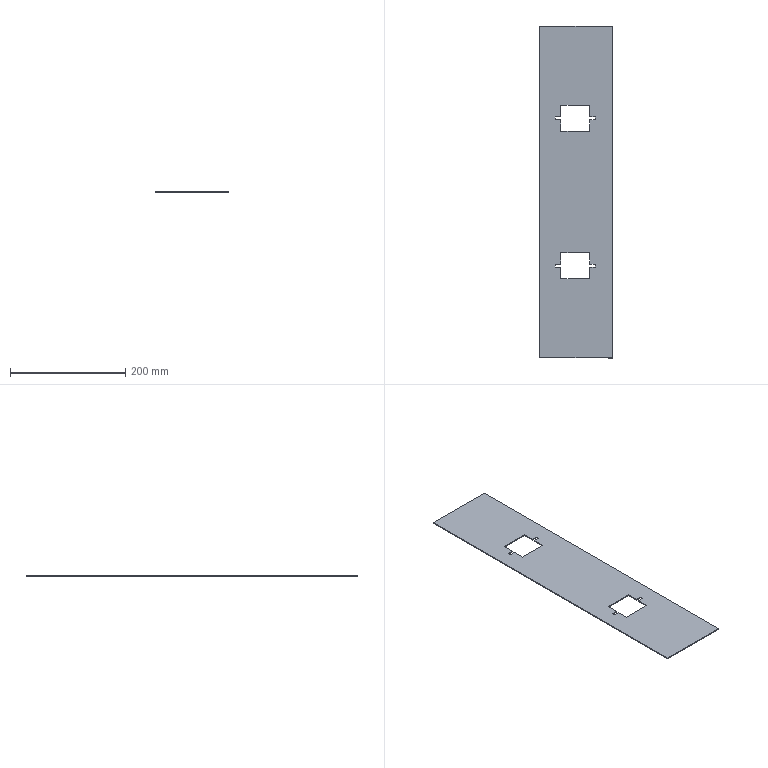Part | SolidWorks | features FlatPattern 1, SMBaseFlange 1, SheetMetal 1 | 1 solid | 30 faces | box 125 x 575 x 1.6 mm | volume 107480 mm3 | plane 30
STEP:
#1=CARTESIAN_POINT('',(-139.19,287.5,1.6));
#2=VERTEX_POINT('',#1);
#3=CARTESIAN_POINT('',(-139.19,-287.5,1.6));
#4=VERTEX_POINT('',#3);
#5=CARTESIAN_POINT('',(-139.19,287.5,1.6));
#6=DIRECTION('',(0.,-1.,0.));
#7=VECTOR('',#6,1000.);
#8=LINE('',#5,#7);
#9=EDGE_CURVE('',#2,#4,#8,.T.);
#10=ORIENTED_EDGE('',*,*,#9,.T.);
#11=CARTESIAN_POINT('',(-14.19,-287.5,1.6));
#12=VERTEX_POINT('',#11);
#13=CARTESIAN_POINT('',(-139.19,-287.5,1.6));
#14=DIRECTION('',(1.,0.,0.));
#15=VECTOR('',#14,1000.);
#16=LINE('',#13,#15);
#17=EDGE_CURVE('',#4,#12,#16,.T.);
#18=ORIENTED_EDGE('',*,*,#17,.T.);
#19=CARTESIAN_POINT('',(-14.19,287.5,1.6));
#20=VERTEX_POINT('',#19);
#21=CARTESIAN_POINT('',(-14.19,287.5,1.6));
#22=DIRECTION('',(0.,1.,0.));
#23=VECTOR('',#22,1000.);
#24=LINE('',#21,#23);
#25=EDGE_CURVE('',#12,#20,#24,.T.);
#26=ORIENTED_EDGE('',*,*,#25,.T.);
#27=CARTESIAN_POINT('',(-139.19,287.5,1.6));
#28=DIRECTION('',(-1.,0.,0.));
#29=VECTOR('',#28,1000.);
#30=LINE('',#27,#29);
#31=EDGE_CURVE('',#20,#2,#30,.T.);
#32=ORIENTED_EDGE('',*,*,#31,.T.);
#33=EDGE_LOOP('',(#10,#18,#26,#32));
#34=FACE_OUTER_BOUND('',#33,.T.);
#35=CARTESIAN_POINT('',(-113.004,-130.,1.6));
#36=VERTEX_POINT('',#35);
#37=CARTESIAN_POINT('',(-103.004,-130.,1.6));
#38=VERTEX_POINT('',#37);
#39=CARTESIAN_POINT('',(-113.004,-130.,1.6));
#40=DIRECTION('',(1.,0.,0.));
#41=VECTOR('',#40,1000.);
#42=LINE('',#39,#41);
#43=EDGE_CURVE('',#36,#38,#42,.T.);
#44=ORIENTED_EDGE('',*,*,#43,.F.);
#45=CARTESIAN_POINT('',(-113.004,-125.,1.6));
#46=VERTEX_POINT('',#45);
#47=CARTESIAN_POINT('',(-113.004,-125.,1.6));
#48=DIRECTION('',(0.,-1.,0.));
#49=VECTOR('',#48,1000.);
#50=LINE('',#47,#49);
#51=EDGE_CURVE('',#46,#36,#50,.T.);
#52=ORIENTED_EDGE('',*,*,#51,.F.);
#53=CARTESIAN_POINT('',(-103.004,-125.,1.6));
#54=VERTEX_POINT('',#53);
#55=CARTESIAN_POINT('',(-113.004,-125.,1.6));
#56=DIRECTION('',(-1.,0.,0.));
#57=VECTOR('',#56,1000.);
#58=LINE('',#55,#57);
#59=EDGE_CURVE('',#54,#46,#58,.T.);
#60=ORIENTED_EDGE('',*,*,#59,.F.);
#61=CARTESIAN_POINT('',(-103.004,-105.,1.6));
#62=VERTEX_POINT('',#61);
#63=CARTESIAN_POINT('',(-103.004,-105.,1.6));
#64=DIRECTION('',(0.,-1.,0.));
#65=VECTOR('',#64,1000.);
#66=LINE('',#63,#65);
#67=EDGE_CURVE('',#62,#54,#66,.T.);
#68=ORIENTED_EDGE('',*,*,#67,.F.);
#69=CARTESIAN_POINT('',(-53.004,-105.,1.6));
#70=VERTEX_POINT('',#69);
#71=CARTESIAN_POINT('',(-103.004,-105.,1.6));
#72=DIRECTION('',(-1.,0.,0.));
#73=VECTOR('',#72,1000.);
#74=LINE('',#71,#73);
#75=EDGE_CURVE('',#70,#62,#74,.T.);
#76=ORIENTED_EDGE('',*,*,#75,.F.);
#77=CARTESIAN_POINT('',(-53.004,-125.,1.6));
#78=VERTEX_POINT('',#77);
#79=CARTESIAN_POINT('',(-53.004,-105.,1.6));
#80=DIRECTION('',(0.,1.,0.));
#81=VECTOR('',#80,1000.);
#82=LINE('',#79,#81);
#83=EDGE_CURVE('',#78,#70,#82,.T.);
#84=ORIENTED_EDGE('',*,*,#83,.F.);
#85=CARTESIAN_POINT('',(-43.004,-125.,1.6));
#86=VERTEX_POINT('',#85);
#87=CARTESIAN_POINT('',(-53.004,-125.,1.6));
#88=DIRECTION('',(-1.,0.,0.));
#89=VECTOR('',#88,1000.);
#90=LINE('',#87,#89);
#91=EDGE_CURVE('',#86,#78,#90,.T.);
#92=ORIENTED_EDGE('',*,*,#91,.F.);
#93=CARTESIAN_POINT('',(-43.004,-130.,1.6));
#94=VERTEX_POINT('',#93);
#95=CARTESIAN_POINT('',(-43.004,-125.,1.6));
#96=DIRECTION('',(0.,1.,0.));
#97=VECTOR('',#96,1000.);
#98=LINE('',#95,#97);
#99=EDGE_CURVE('',#94,#86,#98,.T.);
#100=ORIENTED_EDGE('',*,*,#99,.F.);
#101=CARTESIAN_POINT('',(-53.004,-130.,1.6));
#102=VERTEX_POINT('',#101);
#103=CARTESIAN_POINT('',(-53.004,-130.,1.6));
#104=DIRECTION('',(1.,0.,0.));
#105=VECTOR('',#104,1000.);
#106=LINE('',#103,#105);
#107=EDGE_CURVE('',#102,#94,#106,.T.);
#108=ORIENTED_EDGE('',*,*,#107,.F.);
#109=CARTESIAN_POINT('',(-53.004,-150.,1.6));
#110=VERTEX_POINT('',#109);
#111=CARTESIAN_POINT('',(-53.004,-130.,1.6));
#112=DIRECTION('',(0.,1.,0.));
#113=VECTOR('',#112,1000.);
#114=LINE('',#111,#113);
#115=EDGE_CURVE('',#110,#102,#114,.T.);
#116=ORIENTED_EDGE('',*,*,#115,.F.);
#117=CARTESIAN_POINT('',(-103.004,-150.,1.6));
#118=VERTEX_POINT('',#117);
#119=CARTESIAN_POINT('',(-103.004,-150.,1.6));
#120=DIRECTION('',(1.,0.,0.));
#121=VECTOR('',#120,1000.);
#122=LINE('',#119,#121);
#123=EDGE_CURVE('',#118,#110,#122,.T.);
#124=ORIENTED_EDGE('',*,*,#123,.F.);
#125=CARTESIAN_POINT('',(-103.004,-130.,1.6));
#126=DIRECTION('',(0.,-1.,0.));
#127=VECTOR('',#126,1000.);
#128=LINE('',#125,#127);
#129=EDGE_CURVE('',#38,#118,#128,.T.);
#130=ORIENTED_EDGE('',*,*,#129,.F.);
#131=EDGE_LOOP('',(#44,#52,#60,#68,#76,#84,#92,#100,#108,#116,#124,#130));
#132=FACE_BOUND('',#131,.T.);
#133=CARTESIAN_POINT('',(-53.004,130.,1.6));
#134=VERTEX_POINT('',#133);
#135=CARTESIAN_POINT('',(-53.004,150.,1.6));
#136=VERTEX_POINT('',#135);
#137=CARTESIAN_POINT('',(-53.004,130.,1.6));
#138=DIRECTION('',(0.,1.,0.));
#139=VECTOR('',#138,1000.);
#140=LINE('',#137,#139);
#141=EDGE_CURVE('',#134,#136,#140,.T.);
#142=ORIENTED_EDGE('',*,*,#141,.F.);
#143=CARTESIAN_POINT('',(-43.004,130.,1.6));
#144=VERTEX_POINT('',#143);
#145=CARTESIAN_POINT('',(-53.004,130.,1.6));
#146=DIRECTION('',(-1.,0.,0.));
#147=VECTOR('',#146,1000.);
#148=LINE('',#145,#147);
#149=EDGE_CURVE('',#144,#134,#148,.T.);
#150=ORIENTED_EDGE('',*,*,#149,.F.);
#151=CARTESIAN_POINT('',(-43.004,125.,1.6));
#152=VERTEX_POINT('',#151);
#153=CARTESIAN_POINT('',(-43.004,125.,1.6));
#154=DIRECTION('',(0.,1.,0.));
#155=VECTOR('',#154,1000.);
#156=LINE('',#153,#155);
#157=EDGE_CURVE('',#152,#144,#156,.T.);
#158=ORIENTED_EDGE('',*,*,#157,.F.);
#159=CARTESIAN_POINT('',(-53.004,125.,1.6));
#160=VERTEX_POINT('',#159);
#161=CARTESIAN_POINT('',(-53.004,125.,1.6));
#162=DIRECTION('',(1.,0.,0.));
#163=VECTOR('',#162,1000.);
#164=LINE('',#161,#163);
#165=EDGE_CURVE('',#160,#152,#164,.T.);
#166=ORIENTED_EDGE('',*,*,#165,.F.);
#167=CARTESIAN_POINT('',(-53.004,105.,1.6));
#168=VERTEX_POINT('',#167);
#169=CARTESIAN_POINT('',(-53.004,105.,1.6));
#170=DIRECTION('',(0.,1.,0.));
#171=VECTOR('',#170,1000.);
#172=LINE('',#169,#171);
#173=EDGE_CURVE('',#168,#160,#172,.T.);
#174=ORIENTED_EDGE('',*,*,#173,.F.);
#175=CARTESIAN_POINT('',(-103.004,105.,1.6));
#176=VERTEX_POINT('',#175);
#177=CARTESIAN_POINT('',(-103.004,105.,1.6));
#178=DIRECTION('',(1.,0.,0.));
#179=VECTOR('',#178,1000.);
#180=LINE('',#177,#179);
#181=EDGE_CURVE('',#176,#168,#180,.T.);
#182=ORIENTED_EDGE('',*,*,#181,.F.);
#183=CARTESIAN_POINT('',(-103.004,125.,1.6));
#184=VERTEX_POINT('',#183);
#185=CARTESIAN_POINT('',(-103.004,105.,1.6));
#186=DIRECTION('',(0.,-1.,0.));
#187=VECTOR('',#186,1000.);
#188=LINE('',#185,#187);
#189=EDGE_CURVE('',#184,#176,#188,.T.);
#190=ORIENTED_EDGE('',*,*,#189,.F.);
#191=CARTESIAN_POINT('',(-113.004,125.,1.6));
#192=VERTEX_POINT('',#191);
#193=CARTESIAN_POINT('',(-113.004,125.,1.6));
#194=DIRECTION('',(1.,0.,0.));
#195=VECTOR('',#194,1000.);
#196=LINE('',#193,#195);
#197=EDGE_CURVE('',#192,#184,#196,.T.);
#198=ORIENTED_EDGE('',*,*,#197,.F.);
#199=CARTESIAN_POINT('',(-113.004,130.,1.6));
#200=VERTEX_POINT('',#199);
#201=CARTESIAN_POINT('',(-113.004,125.,1.6));
#202=DIRECTION('',(0.,-1.,0.));
#203=VECTOR('',#202,1000.);
#204=LINE('',#201,#203);
#205=EDGE_CURVE('',#200,#192,#204,.T.);
#206=ORIENTED_EDGE('',*,*,#205,.F.);
#207=CARTESIAN_POINT('',(-103.004,130.,1.6));
#208=VERTEX_POINT('',#207);
#209=CARTESIAN_POINT('',(-113.004,130.,1.6));
#210=DIRECTION('',(-1.,0.,0.));
#211=VECTOR('',#210,1000.);
#212=LINE('',#209,#211);
#213=EDGE_CURVE('',#208,#200,#212,.T.);
#214=ORIENTED_EDGE('',*,*,#213,.F.);
#215=CARTESIAN_POINT('',(-103.004,150.,1.6));
#216=VERTEX_POINT('',#215);
#217=CARTESIAN_POINT('',(-103.004,130.,1.6));
#218=DIRECTION('',(0.,-1.,0.));
#219=VECTOR('',#218,1000.);
#220=LINE('',#217,#219);
#221=EDGE_CURVE('',#216,#208,#220,.T.);
#222=ORIENTED_EDGE('',*,*,#221,.F.);
#223=CARTESIAN_POINT('',(-103.004,150.,1.6));
#224=DIRECTION('',(-1.,0.,0.));
#225=VECTOR('',#224,1000.);
#226=LINE('',#223,#225);
#227=EDGE_CURVE('',#136,#216,#226,.T.);
#228=ORIENTED_EDGE('',*,*,#227,.F.);
#229=EDGE_LOOP('',(#142,#150,#158,#166,#174,#182,#190,#198,#206,#214,#222,#228));
#230=FACE_BOUND('',#229,.T.);
#231=CARTESIAN_POINT('',(0.,0.,1.6));
#232=DIRECTION('',(0.,0.,1.));
#233=DIRECTION('',(1.,0.,0.));
#234=AXIS2_PLACEMENT_3D('',#231,#232,#233);
#235=PLANE('',#234);
#236=ADVANCED_FACE('',(#34,#132,#230),#235,.T.);
#237=CARTESIAN_POINT('',(-113.004,-125.,0.));
#238=VERTEX_POINT('',#237);
#239=CARTESIAN_POINT('',(-113.004,-130.,0.));
#240=VERTEX_POINT('',#239);
#241=CARTESIAN_POINT('',(-113.004,-125.,0.));
#242=DIRECTION('',(0.,-1.,0.));
#243=VECTOR('',#242,1000.);
#244=LINE('',#241,#243);
#245=EDGE_CURVE('',#238,#240,#244,.T.);
#246=ORIENTED_EDGE('',*,*,#245,.T.);
#247=CARTESIAN_POINT('',(-103.004,-130.,0.));
#248=VERTEX_POINT('',#247);
#249=CARTESIAN_POINT('',(-113.004,-130.,0.));
#250=DIRECTION('',(1.,0.,0.));
#251=VECTOR('',#250,1000.);
#252=LINE('',#249,#251);
#253=EDGE_CURVE('',#240,#248,#252,.T.);
#254=ORIENTED_EDGE('',*,*,#253,.T.);
#255=CARTESIAN_POINT('',(-103.004,-150.,0.));
#256=VERTEX_POINT('',#255);
#257=CARTESIAN_POINT('',(-103.004,-130.,0.));
#258=DIRECTION('',(0.,-1.,0.));
#259=VECTOR('',#258,1000.);
#260=LINE('',#257,#259);
#261=EDGE_CURVE('',#248,#256,#260,.T.);
#262=ORIENTED_EDGE('',*,*,#261,.T.);
#263=CARTESIAN_POINT('',(-53.004,-150.,0.));
#264=VERTEX_POINT('',#263);
#265=CARTESIAN_POINT('',(-103.004,-150.,0.));
#266=DIRECTION('',(1.,0.,0.));
#267=VECTOR('',#266,1000.);
#268=LINE('',#265,#267);
#269=EDGE_CURVE('',#256,#264,#268,.T.);
#270=ORIENTED_EDGE('',*,*,#269,.T.);
#271=CARTESIAN_POINT('',(-53.004,-130.,0.));
#272=VERTEX_POINT('',#271);
#273=CARTESIAN_POINT('',(-53.004,-130.,0.));
#274=DIRECTION('',(0.,1.,0.));
#275=VECTOR('',#274,1000.);
#276=LINE('',#273,#275);
#277=EDGE_CURVE('',#264,#272,#276,.T.);
#278=ORIENTED_EDGE('',*,*,#277,.T.);
#279=CARTESIAN_POINT('',(-43.004,-130.,0.));
#280=VERTEX_POINT('',#279);
#281=CARTESIAN_POINT('',(-53.004,-130.,0.));
#282=DIRECTION('',(1.,0.,0.));
#283=VECTOR('',#282,1000.);
#284=LINE('',#281,#283);
#285=EDGE_CURVE('',#272,#280,#284,.T.);
#286=ORIENTED_EDGE('',*,*,#285,.T.);
#287=CARTESIAN_POINT('',(-43.004,-125.,0.));
#288=VERTEX_POINT('',#287);
#289=CARTESIAN_POINT('',(-43.004,-125.,0.));
#290=DIRECTION('',(0.,1.,0.));
#291=VECTOR('',#290,1000.);
#292=LINE('',#289,#291);
#293=EDGE_CURVE('',#280,#288,#292,.T.);
#294=ORIENTED_EDGE('',*,*,#293,.T.);
#295=CARTESIAN_POINT('',(-53.004,-125.,0.));
#296=VERTEX_POINT('',#295);
#297=CARTESIAN_POINT('',(-53.004,-125.,0.));
#298=DIRECTION('',(-1.,0.,0.));
#299=VECTOR('',#298,1000.);
#300=LINE('',#297,#299);
#301=EDGE_CURVE('',#288,#296,#300,.T.);
#302=ORIENTED_EDGE('',*,*,#301,.T.);
#303=CARTESIAN_POINT('',(-53.004,-105.,0.));
#304=VERTEX_POINT('',#303);
#305=CARTESIAN_POINT('',(-53.004,-105.,0.));
#306=DIRECTION('',(0.,1.,0.));
#307=VECTOR('',#306,1000.);
#308=LINE('',#305,#307);
#309=EDGE_CURVE('',#296,#304,#308,.T.);
#310=ORIENTED_EDGE('',*,*,#309,.T.);
#311=CARTESIAN_POINT('',(-103.004,-105.,0.));
#312=VERTEX_POINT('',#311);
#313=CARTESIAN_POINT('',(-103.004,-105.,0.));
#314=DIRECTION('',(-1.,0.,0.));
#315=VECTOR('',#314,1000.);
#316=LINE('',#313,#315);
#317=EDGE_CURVE('',#304,#312,#316,.T.);
#318=ORIENTED_EDGE('',*,*,#317,.T.);
#319=CARTESIAN_POINT('',(-103.004,-125.,0.));
#320=VERTEX_POINT('',#319);
#321=CARTESIAN_POINT('',(-103.004,-105.,0.));
#322=DIRECTION('',(0.,-1.,0.));
#323=VECTOR('',#322,1000.);
#324=LINE('',#321,#323);
#325=EDGE_CURVE('',#312,#320,#324,.T.);
#326=ORIENTED_EDGE('',*,*,#325,.T.);
#327=CARTESIAN_POINT('',(-113.004,-125.,0.));
#328=DIRECTION('',(-1.,0.,0.));
#329=VECTOR('',#328,1000.);
#330=LINE('',#327,#329);
#331=EDGE_CURVE('',#320,#238,#330,.T.);
#332=ORIENTED_EDGE('',*,*,#331,.T.);
#333=EDGE_LOOP('',(#246,#254,#262,#270,#278,#286,#294,#302,#310,#318,#326,#332));
#334=FACE_BOUND('',#333,.T.);
#335=CARTESIAN_POINT('',(-139.19,287.5,0.));
#336=VERTEX_POINT('',#335);
#337=CARTESIAN_POINT('',(-139.19,-287.5,0.));
#338=VERTEX_POINT('',#337);
#339=CARTESIAN_POINT('',(-139.19,287.5,0.));
#340=DIRECTION('',(0.,-1.,0.));
#341=VECTOR('',#340,1000.);
#342=LINE('',#339,#341);
#343=EDGE_CURVE('',#336,#338,#342,.T.);
#344=ORIENTED_EDGE('',*,*,#343,.F.);
#345=CARTESIAN_POINT('',(-14.19,287.5,0.));
#346=VERTEX_POINT('',#345);
#347=CARTESIAN_POINT('',(-139.19,287.5,0.));
#348=DIRECTION('',(-1.,0.,0.));
#349=VECTOR('',#348,1000.);
#350=LINE('',#347,#349);
#351=EDGE_CURVE('',#346,#336,#350,.T.);
#352=ORIENTED_EDGE('',*,*,#351,.F.);
#353=CARTESIAN_POINT('',(-14.19,-287.5,0.));
#354=VERTEX_POINT('',#353);
#355=CARTESIAN_POINT('',(-14.19,287.5,0.));
#356=DIRECTION('',(0.,1.,0.));
#357=VECTOR('',#356,1000.);
#358=LINE('',#355,#357);
#359=EDGE_CURVE('',#354,#346,#358,.T.);
#360=ORIENTED_EDGE('',*,*,#359,.F.);
#361=CARTESIAN_POINT('',(-139.19,-287.5,0.));
#362=DIRECTION('',(1.,0.,0.));
#363=VECTOR('',#362,1000.);
#364=LINE('',#361,#363);
#365=EDGE_CURVE('',#338,#354,#364,.T.);
#366=ORIENTED_EDGE('',*,*,#365,.F.);
#367=EDGE_LOOP('',(#344,#352,#360,#366));
#368=FACE_OUTER_BOUND('',#367,.T.);
#369=CARTESIAN_POINT('',(-43.004,130.,0.));
#370=VERTEX_POINT('',#369);
#371=CARTESIAN_POINT('',(-53.004,130.,0.));
#372=VERTEX_POINT('',#371);
#373=CARTESIAN_POINT('',(-53.004,130.,0.));
#374=DIRECTION('',(-1.,0.,0.));
#375=VECTOR('',#374,1000.);
#376=LINE('',#373,#375);
#377=EDGE_CURVE('',#370,#372,#376,.T.);
#378=ORIENTED_EDGE('',*,*,#377,.T.);
#379=CARTESIAN_POINT('',(-53.004,150.,0.));
#380=VERTEX_POINT('',#379);
#381=CARTESIAN_POINT('',(-53.004,130.,0.));
#382=DIRECTION('',(0.,1.,0.));
#383=VECTOR('',#382,1000.);
#384=LINE('',#381,#383);
#385=EDGE_CURVE('',#372,#380,#384,.T.);
#386=ORIENTED_EDGE('',*,*,#385,.T.);
#387=CARTESIAN_POINT('',(-103.004,150.,0.));
#388=VERTEX_POINT('',#387);
#389=CARTESIAN_POINT('',(-103.004,150.,0.));
#390=DIRECTION('',(-1.,0.,0.));
#391=VECTOR('',#390,1000.);
#392=LINE('',#389,#391);
#393=EDGE_CURVE('',#380,#388,#392,.T.);
#394=ORIENTED_EDGE('',*,*,#393,.T.);
#395=CARTESIAN_POINT('',(-103.004,130.,0.));
#396=VERTEX_POINT('',#395);
#397=CARTESIAN_POINT('',(-103.004,130.,0.));
#398=DIRECTION('',(0.,-1.,0.));
#399=VECTOR('',#398,1000.);
#400=LINE('',#397,#399);
#401=EDGE_CURVE('',#388,#396,#400,.T.);
#402=ORIENTED_EDGE('',*,*,#401,.T.);
#403=CARTESIAN_POINT('',(-113.004,130.,0.));
#404=VERTEX_POINT('',#403);
#405=CARTESIAN_POINT('',(-113.004,130.,0.));
#406=DIRECTION('',(-1.,0.,0.));
#407=VECTOR('',#406,1000.);
#408=LINE('',#405,#407);
#409=EDGE_CURVE('',#396,#404,#408,.T.);
#410=ORIENTED_EDGE('',*,*,#409,.T.);
#411=CARTESIAN_POINT('',(-113.004,125.,0.));
#412=VERTEX_POINT('',#411);
#413=CARTESIAN_POINT('',(-113.004,125.,0.));
#414=DIRECTION('',(0.,-1.,0.));
#415=VECTOR('',#414,1000.);
#416=LINE('',#413,#415);
#417=EDGE_CURVE('',#404,#412,#416,.T.);
#418=ORIENTED_EDGE('',*,*,#417,.T.);
#419=CARTESIAN_POINT('',(-103.004,125.,0.));
#420=VERTEX_POINT('',#419);
#421=CARTESIAN_POINT('',(-113.004,125.,0.));
#422=DIRECTION('',(1.,0.,0.));
#423=VECTOR('',#422,1000.);
#424=LINE('',#421,#423);
#425=EDGE_CURVE('',#412,#420,#424,.T.);
#426=ORIENTED_EDGE('',*,*,#425,.T.);
#427=CARTESIAN_POINT('',(-103.004,105.,0.));
#428=VERTEX_POINT('',#427);
#429=CARTESIAN_POINT('',(-103.004,105.,0.));
#430=DIRECTION('',(0.,-1.,0.));
#431=VECTOR('',#430,1000.);
#432=LINE('',#429,#431);
#433=EDGE_CURVE('',#420,#428,#432,.T.);
#434=ORIENTED_EDGE('',*,*,#433,.T.);
#435=CARTESIAN_POINT('',(-53.004,105.,0.));
#436=VERTEX_POINT('',#435);
#437=CARTESIAN_POINT('',(-103.004,105.,0.));
#438=DIRECTION('',(1.,0.,0.));
#439=VECTOR('',#438,1000.);
#440=LINE('',#437,#439);
#441=EDGE_CURVE('',#428,#436,#440,.T.);
#442=ORIENTED_EDGE('',*,*,#441,.T.);
#443=CARTESIAN_POINT('',(-53.004,125.,0.));
#444=VERTEX_POINT('',#443);
#445=CARTESIAN_POINT('',(-53.004,105.,0.));
#446=DIRECTION('',(0.,1.,0.));
#447=VECTOR('',#446,1000.);
#448=LINE('',#445,#447);
#449=EDGE_CURVE('',#436,#444,#448,.T.);
#450=ORIENTED_EDGE('',*,*,#449,.T.);
#451=CARTESIAN_POINT('',(-43.004,125.,0.));
#452=VERTEX_POINT('',#451);
#453=CARTESIAN_POINT('',(-53.004,125.,0.));
#454=DIRECTION('',(1.,0.,0.));
#455=VECTOR('',#454,1000.);
#456=LINE('',#453,#455);
#457=EDGE_CURVE('',#444,#452,#456,.T.);
#458=ORIENTED_EDGE('',*,*,#457,.T.);
#459=CARTESIAN_POINT('',(-43.004,125.,0.));
#460=DIRECTION('',(0.,1.,0.));
#461=VECTOR('',#460,1000.);
#462=LINE('',#459,#461);
#463=EDGE_CURVE('',#452,#370,#462,.T.);
#464=ORIENTED_EDGE('',*,*,#463,.T.);
#465=EDGE_LOOP('',(#378,#386,#394,#402,#410,#418,#426,#434,#442,#450,#458,#464));
#466=FACE_BOUND('',#465,.T.);
#467=CARTESIAN_POINT('',(0.,0.,0.));
#468=DIRECTION('',(0.,0.,1.));
#469=DIRECTION('',(1.,0.,0.));
#470=AXIS2_PLACEMENT_3D('',#467,#468,#469);
#471=PLANE('',#470);
#472=ADVANCED_FACE('',(#334,#368,#466),#471,.F.);
#473=ORIENTED_EDGE('',*,*,#343,.T.);
#474=CARTESIAN_POINT('',(-139.19,-287.5,1.6));
#475=DIRECTION('',(0.,0.,-1.));
#476=VECTOR('',#475,1000.);
#477=LINE('',#474,#476);
#478=EDGE_CURVE('',#4,#338,#477,.T.);
#479=ORIENTED_EDGE('',*,*,#478,.F.);
#480=ORIENTED_EDGE('',*,*,#9,.F.);
#481=CARTESIAN_POINT('',(-139.19,287.5,1.6));
#482=DIRECTION('',(0.,0.,-1.));
#483=VECTOR('',#482,1000.);
#484=LINE('',#481,#483);
#485=EDGE_CURVE('',#2,#336,#484,.T.);
#486=ORIENTED_EDGE('',*,*,#485,.T.);
#487=EDGE_LOOP('',(#473,#479,#480,#486));
#488=FACE_OUTER_BOUND('',#487,.T.);
#489=CARTESIAN_POINT('',(-139.19,287.5,1.6));
#490=DIRECTION('',(1.,0.,0.));
#491=DIRECTION('',(0.,0.,-1.));
#492=AXIS2_PLACEMENT_3D('',#489,#490,#491);
#493=PLANE('',#492);
#494=ADVANCED_FACE('',(#488),#493,.F.);
#495=ORIENTED_EDGE('',*,*,#365,.T.);
#496=CARTESIAN_POINT('',(-14.19,-287.5,1.6));
#497=DIRECTION('',(0.,0.,-1.));
#498=VECTOR('',#497,1000.);
#499=LINE('',#496,#498);
#500=EDGE_CURVE('',#12,#354,#499,.T.);
#501=ORIENTED_EDGE('',*,*,#500,.F.);
#502=ORIENTED_EDGE('',*,*,#17,.F.);
#503=ORIENTED_EDGE('',*,*,#478,.T.);
#504=EDGE_LOOP('',(#495,#501,#502,#503));
#505=FACE_OUTER_BOUND('',#504,.T.);
#506=CARTESIAN_POINT('',(-139.19,-287.5,1.6));
#507=DIRECTION('',(0.,1.,0.));
#508=DIRECTION('',(-1.,0.,0.));
#509=AXIS2_PLACEMENT_3D('',#506,#507,#508);
#510=PLANE('',#509);
#511=ADVANCED_FACE('',(#505),#510,.F.);
#512=ORIENTED_EDGE('',*,*,#359,.T.);
#513=CARTESIAN_POINT('',(-14.19,287.5,1.6));
#514=DIRECTION('',(0.,0.,-1.));
#515=VECTOR('',#514,1000.);
#516=LINE('',#513,#515);
#517=EDGE_CURVE('',#20,#346,#516,.T.);
#518=ORIENTED_EDGE('',*,*,#517,.F.);
#519=ORIENTED_EDGE('',*,*,#25,.F.);
#520=ORIENTED_EDGE('',*,*,#500,.T.);
#521=EDGE_LOOP('',(#512,#518,#519,#520));
#522=FACE_OUTER_BOUND('',#521,.T.);
#523=CARTESIAN_POINT('',(-14.19,287.5,1.6));
#524=DIRECTION('',(-1.,0.,0.));
#525=DIRECTION('',(0.,-1.,0.));
#526=AXIS2_PLACEMENT_3D('',#523,#524,#525);
#527=PLANE('',#526);
#528=ADVANCED_FACE('',(#522),#527,.F.);
#529=ORIENTED_EDGE('',*,*,#351,.T.);
#530=ORIENTED_EDGE('',*,*,#485,.F.);
#531=ORIENTED_EDGE('',*,*,#31,.F.);
#532=ORIENTED_EDGE('',*,*,#517,.T.);
#533=EDGE_LOOP('',(#529,#530,#531,#532));
#534=FACE_OUTER_BOUND('',#533,.T.);
#535=CARTESIAN_POINT('',(-139.19,287.5,1.6));
#536=DIRECTION('',(0.,-1.,0.));
#537=DIRECTION('',(0.,0.,-1.));
#538=AXIS2_PLACEMENT_3D('',#535,#536,#537);
#539=PLANE('',#538);
#540=ADVANCED_FACE('',(#534),#539,.F.);
#541=ORIENTED_EDGE('',*,*,#245,.F.);
#542=CARTESIAN_POINT('',(-113.004,-125.,1.6));
#543=DIRECTION('',(0.,0.,-1.));
#544=VECTOR('',#543,1000.);
#545=LINE('',#542,#544);
#546=EDGE_CURVE('',#46,#238,#545,.T.);
#547=ORIENTED_EDGE('',*,*,#546,.F.);
#548=ORIENTED_EDGE('',*,*,#51,.T.);
#549=CARTESIAN_POINT('',(-113.004,-130.,1.6));
#550=DIRECTION('',(0.,0.,-1.));
#551=VECTOR('',#550,1000.);
#552=LINE('',#549,#551);
#553=EDGE_CURVE('',#36,#240,#552,.T.);
#554=ORIENTED_EDGE('',*,*,#553,.T.);
#555=EDGE_LOOP('',(#541,#547,#548,#554));
#556=FACE_OUTER_BOUND('',#555,.T.);
#557=CARTESIAN_POINT('',(-113.004,-125.,1.6));
#558=DIRECTION('',(1.,0.,0.));
#559=DIRECTION('',(0.,0.,-1.));
#560=AXIS2_PLACEMENT_3D('',#557,#558,#559);
#561=PLANE('',#560);
#562=ADVANCED_FACE('',(#556),#561,.T.);
#563=ORIENTED_EDGE('',*,*,#253,.F.);
#564=ORIENTED_EDGE('',*,*,#553,.F.);
#565=ORIENTED_EDGE('',*,*,#43,.T.);
#566=CARTESIAN_POINT('',(-103.004,-130.,1.6));
#567=DIRECTION('',(0.,0.,-1.));
#568=VECTOR('',#567,1000.);
#569=LINE('',#566,#568);
#570=EDGE_CURVE('',#38,#248,#569,.T.);
#571=ORIENTED_EDGE('',*,*,#570,.T.);
#572=EDGE_LOOP('',(#563,#564,#565,#571));
#573=FACE_OUTER_BOUND('',#572,.T.);
#574=CARTESIAN_POINT('',(-113.004,-130.,1.6));
#575=DIRECTION('',(0.,1.,0.));
#576=DIRECTION('',(0.,0.,1.));
#577=AXIS2_PLACEMENT_3D('',#574,#575,#576);
#578=PLANE('',#577);
#579=ADVANCED_FACE('',(#573),#578,.T.);
#580=ORIENTED_EDGE('',*,*,#261,.F.);
#581=ORIENTED_EDGE('',*,*,#570,.F.);
#582=ORIENTED_EDGE('',*,*,#129,.T.);
#583=CARTESIAN_POINT('',(-103.004,-150.,1.6));
#584=DIRECTION('',(0.,0.,-1.));
#585=VECTOR('',#584,1000.);
#586=LINE('',#583,#585);
#587=EDGE_CURVE('',#118,#256,#586,.T.);
#588=ORIENTED_EDGE('',*,*,#587,.T.);
#589=EDGE_LOOP('',(#580,#581,#582,#588));
#590=FACE_OUTER_BOUND('',#589,.T.);
#591=CARTESIAN_POINT('',(-103.004,-130.,1.6));
#592=DIRECTION('',(1.,0.,0.));
#593=DIRECTION('',(0.,0.,-1.));
#594=AXIS2_PLACEMENT_3D('',#591,#592,#593);
#595=PLANE('',#594);
#596=ADVANCED_FACE('',(#590),#595,.T.);
#597=ORIENTED_EDGE('',*,*,#269,.F.);
#598=ORIENTED_EDGE('',*,*,#587,.F.);
#599=ORIENTED_EDGE('',*,*,#123,.T.);
#600=CARTESIAN_POINT('',(-53.004,-150.,1.6));
#601=DIRECTION('',(0.,0.,-1.));
#602=VECTOR('',#601,1000.);
#603=LINE('',#600,#602);
#604=EDGE_CURVE('',#110,#264,#603,.T.);
#605=ORIENTED_EDGE('',*,*,#604,.T.);
#606=EDGE_LOOP('',(#597,#598,#599,#605));
#607=FACE_OUTER_BOUND('',#606,.T.);
#608=CARTESIAN_POINT('',(-103.004,-150.,1.6));
#609=DIRECTION('',(0.,1.,0.));
#610=DIRECTION('',(0.,0.,1.));
#611=AXIS2_PLACEMENT_3D('',#608,#609,#610);
#612=PLANE('',#611);
#613=ADVANCED_FACE('',(#607),#612,.T.);
#614=ORIENTED_EDGE('',*,*,#277,.F.);
#615=ORIENTED_EDGE('',*,*,#604,.F.);
#616=ORIENTED_EDGE('',*,*,#115,.T.);
#617=CARTESIAN_POINT('',(-53.004,-130.,1.6));
#618=DIRECTION('',(0.,0.,-1.));
#619=VECTOR('',#618,1000.);
#620=LINE('',#617,#619);
#621=EDGE_CURVE('',#102,#272,#620,.T.);
#622=ORIENTED_EDGE('',*,*,#621,.T.);
#623=EDGE_LOOP('',(#614,#615,#616,#622));
#624=FACE_OUTER_BOUND('',#623,.T.);
#625=CARTESIAN_POINT('',(-53.004,-130.,1.6));
#626=DIRECTION('',(-1.,0.,0.));
#627=DIRECTION('',(0.,0.,1.));
#628=AXIS2_PLACEMENT_3D('',#625,#626,#627);
#629=PLANE('',#628);
#630=ADVANCED_FACE('',(#624),#629,.T.);
#631=ORIENTED_EDGE('',*,*,#285,.F.);
#632=ORIENTED_EDGE('',*,*,#621,.F.);
#633=ORIENTED_EDGE('',*,*,#107,.T.);
#634=CARTESIAN_POINT('',(-43.004,-130.,1.6));
#635=DIRECTION('',(0.,0.,-1.));
#636=VECTOR('',#635,1000.);
#637=LINE('',#634,#636);
#638=EDGE_CURVE('',#94,#280,#637,.T.);
#639=ORIENTED_EDGE('',*,*,#638,.T.);
#640=EDGE_LOOP('',(#631,#632,#633,#639));
#641=FACE_OUTER_BOUND('',#640,.T.);
#642=CARTESIAN_POINT('',(-53.004,-130.,1.6));
#643=DIRECTION('',(0.,1.,0.));
#644=DIRECTION('',(0.,0.,1.));
#645=AXIS2_PLACEMENT_3D('',#642,#643,#644);
#646=PLANE('',#645);
#647=ADVANCED_FACE('',(#641),#646,.T.);
#648=ORIENTED_EDGE('',*,*,#293,.F.);
#649=ORIENTED_EDGE('',*,*,#638,.F.);
#650=ORIENTED_EDGE('',*,*,#99,.T.);
#651=CARTESIAN_POINT('',(-43.004,-125.,1.6));
#652=DIRECTION('',(0.,0.,-1.));
#653=VECTOR('',#652,1000.);
#654=LINE('',#651,#653);
#655=EDGE_CURVE('',#86,#288,#654,.T.);
#656=ORIENTED_EDGE('',*,*,#655,.T.);
#657=EDGE_LOOP('',(#648,#649,#650,#656));
#658=FACE_OUTER_BOUND('',#657,.T.);
#659=CARTESIAN_POINT('',(-43.004,-125.,1.6));
#660=DIRECTION('',(-1.,0.,0.));
#661=DIRECTION('',(0.,0.,1.));
#662=AXIS2_PLACEMENT_3D('',#659,#660,#661);
#663=PLANE('',#662);
#664=ADVANCED_FACE('',(#658),#663,.T.);
#665=ORIENTED_EDGE('',*,*,#301,.F.);
#666=ORIENTED_EDGE('',*,*,#655,.F.);
#667=ORIENTED_EDGE('',*,*,#91,.T.);
#668=CARTESIAN_POINT('',(-53.004,-125.,1.6));
#669=DIRECTION('',(0.,0.,-1.));
#670=VECTOR('',#669,1000.);
#671=LINE('',#668,#670);
#672=EDGE_CURVE('',#78,#296,#671,.T.);
#673=ORIENTED_EDGE('',*,*,#672,.T.);
#674=EDGE_LOOP('',(#665,#666,#667,#673));
#675=FACE_OUTER_BOUND('',#674,.T.);
#676=CARTESIAN_POINT('',(-53.004,-125.,1.6));
#677=DIRECTION('',(0.,-1.,0.));
#678=DIRECTION('',(0.,0.,-1.));
#679=AXIS2_PLACEMENT_3D('',#676,#677,#678);
#680=PLANE('',#679);
#681=ADVANCED_FACE('',(#675),#680,.T.);
#682=ORIENTED_EDGE('',*,*,#309,.F.);
#683=ORIENTED_EDGE('',*,*,#672,.F.);
#684=ORIENTED_EDGE('',*,*,#83,.T.);
#685=CARTESIAN_POINT('',(-53.004,-105.,1.6));
#686=DIRECTION('',(0.,0.,-1.));
#687=VECTOR('',#686,1000.);
#688=LINE('',#685,#687);
#689=EDGE_CURVE('',#70,#304,#688,.T.);
#690=ORIENTED_EDGE('',*,*,#689,.T.);
#691=EDGE_LOOP('',(#682,#683,#684,#690));
#692=FACE_OUTER_BOUND('',#691,.T.);
#693=CARTESIAN_POINT('',(-53.004,-105.,1.6));
#694=DIRECTION('',(-1.,0.,0.));
#695=DIRECTION('',(0.,0.,1.));
#696=AXIS2_PLACEMENT_3D('',#693,#694,#695);
#697=PLANE('',#696);
#698=ADVANCED_FACE('',(#692),#697,.T.);
#699=ORIENTED_EDGE('',*,*,#317,.F.);
#700=ORIENTED_EDGE('',*,*,#689,.F.);
#701=ORIENTED_EDGE('',*,*,#75,.T.);
#702=CARTESIAN_POINT('',(-103.004,-105.,1.6));
#703=DIRECTION('',(0.,0.,-1.));
#704=VECTOR('',#703,1000.);
#705=LINE('',#702,#704);
#706=EDGE_CURVE('',#62,#312,#705,.T.);
#707=ORIENTED_EDGE('',*,*,#706,.T.);
#708=EDGE_LOOP('',(#699,#700,#701,#707));
#709=FACE_OUTER_BOUND('',#708,.T.);
#710=CARTESIAN_POINT('',(-103.004,-105.,1.6));
#711=DIRECTION('',(0.,-1.,0.));
#712=DIRECTION('',(0.,0.,-1.));
#713=AXIS2_PLACEMENT_3D('',#710,#711,#712);
#714=PLANE('',#713);
#715=ADVANCED_FACE('',(#709),#714,.T.);
#716=ORIENTED_EDGE('',*,*,#325,.F.);
#717=ORIENTED_EDGE('',*,*,#706,.F.);
#718=ORIENTED_EDGE('',*,*,#67,.T.);
#719=CARTESIAN_POINT('',(-103.004,-125.,1.6));
#720=DIRECTION('',(0.,0.,-1.));
#721=VECTOR('',#720,1000.);
#722=LINE('',#719,#721);
#723=EDGE_CURVE('',#54,#320,#722,.T.);
#724=ORIENTED_EDGE('',*,*,#723,.T.);
#725=EDGE_LOOP('',(#716,#717,#718,#724));
#726=FACE_OUTER_BOUND('',#725,.T.);
#727=CARTESIAN_POINT('',(-103.004,-105.,1.6));
#728=DIRECTION('',(1.,0.,0.));
#729=DIRECTION('',(0.,0.,-1.));
#730=AXIS2_PLACEMENT_3D('',#727,#728,#729);
#731=PLANE('',#730);
#732=ADVANCED_FACE('',(#726),#731,.T.);
#733=ORIENTED_EDGE('',*,*,#331,.F.);
#734=ORIENTED_EDGE('',*,*,#723,.F.);
#735=ORIENTED_EDGE('',*,*,#59,.T.);
#736=ORIENTED_EDGE('',*,*,#546,.T.);
#737=EDGE_LOOP('',(#733,#734,#735,#736));
#738=FACE_OUTER_BOUND('',#737,.T.);
#739=CARTESIAN_POINT('',(-113.004,-125.,1.6));
#740=DIRECTION('',(0.,-1.,0.));
#741=DIRECTION('',(0.,0.,-1.));
#742=AXIS2_PLACEMENT_3D('',#739,#740,#741);
#743=PLANE('',#742);
#744=ADVANCED_FACE('',(#738),#743,.T.);
#745=ORIENTED_EDGE('',*,*,#377,.F.);
#746=CARTESIAN_POINT('',(-43.004,130.,1.6));
#747=DIRECTION('',(0.,0.,-1.));
#748=VECTOR('',#747,1000.);
#749=LINE('',#746,#748);
#750=EDGE_CURVE('',#144,#370,#749,.T.);
#751=ORIENTED_EDGE('',*,*,#750,.F.);
#752=ORIENTED_EDGE('',*,*,#149,.T.);
#753=CARTESIAN_POINT('',(-53.004,130.,1.6));
#754=DIRECTION('',(0.,0.,-1.));
#755=VECTOR('',#754,1000.);
#756=LINE('',#753,#755);
#757=EDGE_CURVE('',#134,#372,#756,.T.);
#758=ORIENTED_EDGE('',*,*,#757,.T.);
#759=EDGE_LOOP('',(#745,#751,#752,#758));
#760=FACE_OUTER_BOUND('',#759,.T.);
#761=CARTESIAN_POINT('',(-53.004,130.,1.6));
#762=DIRECTION('',(0.,-1.,0.));
#763=DIRECTION('',(0.,0.,-1.));
#764=AXIS2_PLACEMENT_3D('',#761,#762,#763);
#765=PLANE('',#764);
#766=ADVANCED_FACE('',(#760),#765,.T.);
#767=ORIENTED_EDGE('',*,*,#385,.F.);
#768=ORIENTED_EDGE('',*,*,#757,.F.);
#769=ORIENTED_EDGE('',*,*,#141,.T.);
#770=CARTESIAN_POINT('',(-53.004,150.,1.6));
#771=DIRECTION('',(0.,0.,-1.));
#772=VECTOR('',#771,1000.);
#773=LINE('',#770,#772);
#774=EDGE_CURVE('',#136,#380,#773,.T.);
#775=ORIENTED_EDGE('',*,*,#774,.T.);
#776=EDGE_LOOP('',(#767,#768,#769,#775));
#777=FACE_OUTER_BOUND('',#776,.T.);
#778=CARTESIAN_POINT('',(-53.004,130.,1.6));
#779=DIRECTION('',(-1.,0.,0.));
#780=DIRECTION('',(0.,0.,1.));
#781=AXIS2_PLACEMENT_3D('',#778,#779,#780);
#782=PLANE('',#781);
#783=ADVANCED_FACE('',(#777),#782,.T.);
#784=ORIENTED_EDGE('',*,*,#393,.F.);
#785=ORIENTED_EDGE('',*,*,#774,.F.);
#786=ORIENTED_EDGE('',*,*,#227,.T.);
#787=CARTESIAN_POINT('',(-103.004,150.,1.6));
#788=DIRECTION('',(0.,0.,-1.));
#789=VECTOR('',#788,1000.);
#790=LINE('',#787,#789);
#791=EDGE_CURVE('',#216,#388,#790,.T.);
#792=ORIENTED_EDGE('',*,*,#791,.T.);
#793=EDGE_LOOP('',(#784,#785,#786,#792));
#794=FACE_OUTER_BOUND('',#793,.T.);
#795=CARTESIAN_POINT('',(-103.004,150.,1.6));
#796=DIRECTION('',(0.,-1.,0.));
#797=DIRECTION('',(0.,0.,-1.));
#798=AXIS2_PLACEMENT_3D('',#795,#796,#797);
#799=PLANE('',#798);
#800=ADVANCED_FACE('',(#794),#799,.T.);
#801=ORIENTED_EDGE('',*,*,#401,.F.);
#802=ORIENTED_EDGE('',*,*,#791,.F.);
#803=ORIENTED_EDGE('',*,*,#221,.T.);
#804=CARTESIAN_POINT('',(-103.004,130.,1.6));
#805=DIRECTION('',(0.,0.,-1.));
#806=VECTOR('',#805,1000.);
#807=LINE('',#804,#806);
#808=EDGE_CURVE('',#208,#396,#807,.T.);
#809=ORIENTED_EDGE('',*,*,#808,.T.);
#810=EDGE_LOOP('',(#801,#802,#803,#809));
#811=FACE_OUTER_BOUND('',#810,.T.);
#812=CARTESIAN_POINT('',(-103.004,130.,1.6));
#813=DIRECTION('',(1.,0.,0.));
#814=DIRECTION('',(0.,0.,-1.));
#815=AXIS2_PLACEMENT_3D('',#812,#813,#814);
#816=PLANE('',#815);
#817=ADVANCED_FACE('',(#811),#816,.T.);
#818=ORIENTED_EDGE('',*,*,#409,.F.);
#819=ORIENTED_EDGE('',*,*,#808,.F.);
#820=ORIENTED_EDGE('',*,*,#213,.T.);
#821=CARTESIAN_POINT('',(-113.004,130.,1.6));
#822=DIRECTION('',(0.,0.,-1.));
#823=VECTOR('',#822,1000.);
#824=LINE('',#821,#823);
#825=EDGE_CURVE('',#200,#404,#824,.T.);
#826=ORIENTED_EDGE('',*,*,#825,.T.);
#827=EDGE_LOOP('',(#818,#819,#820,#826));
#828=FACE_OUTER_BOUND('',#827,.T.);
#829=CARTESIAN_POINT('',(-113.004,130.,1.6));
#830=DIRECTION('',(0.,-1.,0.));
#831=DIRECTION('',(0.,0.,-1.));
#832=AXIS2_PLACEMENT_3D('',#829,#830,#831);
#833=PLANE('',#832);
#834=ADVANCED_FACE('',(#828),#833,.T.);
#835=ORIENTED_EDGE('',*,*,#417,.F.);
#836=ORIENTED_EDGE('',*,*,#825,.F.);
#837=ORIENTED_EDGE('',*,*,#205,.T.);
#838=CARTESIAN_POINT('',(-113.004,125.,1.6));
#839=DIRECTION('',(0.,0.,-1.));
#840=VECTOR('',#839,1000.);
#841=LINE('',#838,#840);
#842=EDGE_CURVE('',#192,#412,#841,.T.);
#843=ORIENTED_EDGE('',*,*,#842,.T.);
#844=EDGE_LOOP('',(#835,#836,#837,#843));
#845=FACE_OUTER_BOUND('',#844,.T.);
#846=CARTESIAN_POINT('',(-113.004,125.,1.6));
#847=DIRECTION('',(1.,0.,0.));
#848=DIRECTION('',(0.,0.,-1.));
#849=AXIS2_PLACEMENT_3D('',#846,#847,#848);
#850=PLANE('',#849);
#851=ADVANCED_FACE('',(#845),#850,.T.);
#852=ORIENTED_EDGE('',*,*,#425,.F.);
#853=ORIENTED_EDGE('',*,*,#842,.F.);
#854=ORIENTED_EDGE('',*,*,#197,.T.);
#855=CARTESIAN_POINT('',(-103.004,125.,1.6));
#856=DIRECTION('',(0.,0.,-1.));
#857=VECTOR('',#856,1000.);
#858=LINE('',#855,#857);
#859=EDGE_CURVE('',#184,#420,#858,.T.);
#860=ORIENTED_EDGE('',*,*,#859,.T.);
#861=EDGE_LOOP('',(#852,#853,#854,#860));
#862=FACE_OUTER_BOUND('',#861,.T.);
#863=CARTESIAN_POINT('',(-113.004,125.,1.6));
#864=DIRECTION('',(0.,1.,0.));
#865=DIRECTION('',(0.,0.,1.));
#866=AXIS2_PLACEMENT_3D('',#863,#864,#865);
#867=PLANE('',#866);
#868=ADVANCED_FACE('',(#862),#867,.T.);
#869=ORIENTED_EDGE('',*,*,#433,.F.);
#870=ORIENTED_EDGE('',*,*,#859,.F.);
#871=ORIENTED_EDGE('',*,*,#189,.T.);
#872=CARTESIAN_POINT('',(-103.004,105.,1.6));
#873=DIRECTION('',(0.,0.,-1.));
#874=VECTOR('',#873,1000.);
#875=LINE('',#872,#874);
#876=EDGE_CURVE('',#176,#428,#875,.T.);
#877=ORIENTED_EDGE('',*,*,#876,.T.);
#878=EDGE_LOOP('',(#869,#870,#871,#877));
#879=FACE_OUTER_BOUND('',#878,.T.);
#880=CARTESIAN_POINT('',(-103.004,105.,1.6));
#881=DIRECTION('',(1.,0.,0.));
#882=DIRECTION('',(0.,0.,-1.));
#883=AXIS2_PLACEMENT_3D('',#880,#881,#882);
#884=PLANE('',#883);
#885=ADVANCED_FACE('',(#879),#884,.T.);
#886=ORIENTED_EDGE('',*,*,#441,.F.);
#887=ORIENTED_EDGE('',*,*,#876,.F.);
#888=ORIENTED_EDGE('',*,*,#181,.T.);
#889=CARTESIAN_POINT('',(-53.004,105.,1.6));
#890=DIRECTION('',(0.,0.,-1.));
#891=VECTOR('',#890,1000.);
#892=LINE('',#889,#891);
#893=EDGE_CURVE('',#168,#436,#892,.T.);
#894=ORIENTED_EDGE('',*,*,#893,.T.);
#895=EDGE_LOOP('',(#886,#887,#888,#894));
#896=FACE_OUTER_BOUND('',#895,.T.);
#897=CARTESIAN_POINT('',(-103.004,105.,1.6));
#898=DIRECTION('',(0.,1.,0.));
#899=DIRECTION('',(0.,0.,1.));
#900=AXIS2_PLACEMENT_3D('',#897,#898,#899);
#901=PLANE('',#900);
#902=ADVANCED_FACE('',(#896),#901,.T.);
#903=ORIENTED_EDGE('',*,*,#449,.F.);
#904=ORIENTED_EDGE('',*,*,#893,.F.);
#905=ORIENTED_EDGE('',*,*,#173,.T.);
#906=CARTESIAN_POINT('',(-53.004,125.,1.6));
#907=DIRECTION('',(0.,0.,-1.));
#908=VECTOR('',#907,1000.);
#909=LINE('',#906,#908);
#910=EDGE_CURVE('',#160,#444,#909,.T.);
#911=ORIENTED_EDGE('',*,*,#910,.T.);
#912=EDGE_LOOP('',(#903,#904,#905,#911));
#913=FACE_OUTER_BOUND('',#912,.T.);
#914=CARTESIAN_POINT('',(-53.004,105.,1.6));
#915=DIRECTION('',(-1.,0.,0.));
#916=DIRECTION('',(0.,0.,1.));
#917=AXIS2_PLACEMENT_3D('',#914,#915,#916);
#918=PLANE('',#917);
#919=ADVANCED_FACE('',(#913),#918,.T.);
#920=ORIENTED_EDGE('',*,*,#457,.F.);
#921=ORIENTED_EDGE('',*,*,#910,.F.);
#922=ORIENTED_EDGE('',*,*,#165,.T.);
#923=CARTESIAN_POINT('',(-43.004,125.,1.6));
#924=DIRECTION('',(0.,0.,-1.));
#925=VECTOR('',#924,1000.);
#926=LINE('',#923,#925);
#927=EDGE_CURVE('',#152,#452,#926,.T.);
#928=ORIENTED_EDGE('',*,*,#927,.T.);
#929=EDGE_LOOP('',(#920,#921,#922,#928));
#930=FACE_OUTER_BOUND('',#929,.T.);
#931=CARTESIAN_POINT('',(-53.004,125.,1.6));
#932=DIRECTION('',(0.,1.,0.));
#933=DIRECTION('',(0.,0.,1.));
#934=AXIS2_PLACEMENT_3D('',#931,#932,#933);
#935=PLANE('',#934);
#936=ADVANCED_FACE('',(#930),#935,.T.);
#937=ORIENTED_EDGE('',*,*,#463,.F.);
#938=ORIENTED_EDGE('',*,*,#927,.F.);
#939=ORIENTED_EDGE('',*,*,#157,.T.);
#940=ORIENTED_EDGE('',*,*,#750,.T.);
#941=EDGE_LOOP('',(#937,#938,#939,#940));
#942=FACE_OUTER_BOUND('',#941,.T.);
#943=CARTESIAN_POINT('',(-43.004,125.,1.6));
#944=DIRECTION('',(-1.,0.,0.));
#945=DIRECTION('',(0.,0.,1.));
#946=AXIS2_PLACEMENT_3D('',#943,#944,#945);
#947=PLANE('',#946);
#948=ADVANCED_FACE('',(#942),#947,.T.);
#949=CLOSED_SHELL('',(#236,#472,#494,#511,#528,#540,#562,#579,#596,#613,#630,#647,#664,#681,#698,#715,#732,#744,#766,#783,#800,#817,#834,#851,#868,#885,#902,#919,#936,#948));
#950=MANIFOLD_SOLID_BREP('',#949);
#951=CARTESIAN_POINT('',(0.,0.,0.));
#952=DIRECTION('',(0.,0.,1.));
#953=DIRECTION('',(1.,0.,0.));
#954=AXIS2_PLACEMENT_3D('',#951,#952,#953);
#955=(LENGTH_UNIT()NAMED_UNIT(*)SI_UNIT(.MILLI.,.METRE.));
#956=UNCERTAINTY_MEASURE_WITH_UNIT(LENGTH_MEASURE(0.00001),#955,'','');
#957=(NAMED_UNIT(*)PLANE_ANGLE_UNIT()SI_UNIT($,.RADIAN.));
#958=(NAMED_UNIT(*)SI_UNIT($,.STERADIAN.)SOLID_ANGLE_UNIT());
#959=(GEOMETRIC_REPRESENTATION_CONTEXT(3)GLOBAL_UNCERTAINTY_ASSIGNED_CONTEXT((#956))GLOBAL_UNIT_ASSIGNED_CONTEXT((#955,#957,#958))REPRESENTATION_CONTEXT('',''));
#960=ADVANCED_BREP_SHAPE_REPRESENTATION('',(#950,#954),#959);